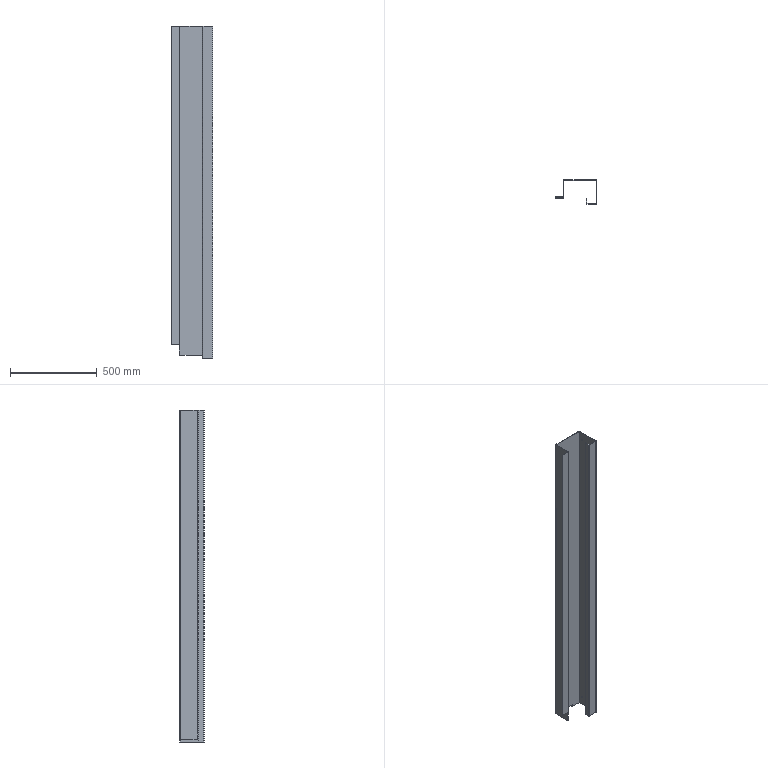Part | STEP file | TS-S102 | 1 solid | 56 faces | box 240 x 140 x 1910 mm | volume 3171467 mm3 | plane 38 | cylinder 18 | commonest cylinder face diameters 5.4 x8 0.4 x5 6.4 x5